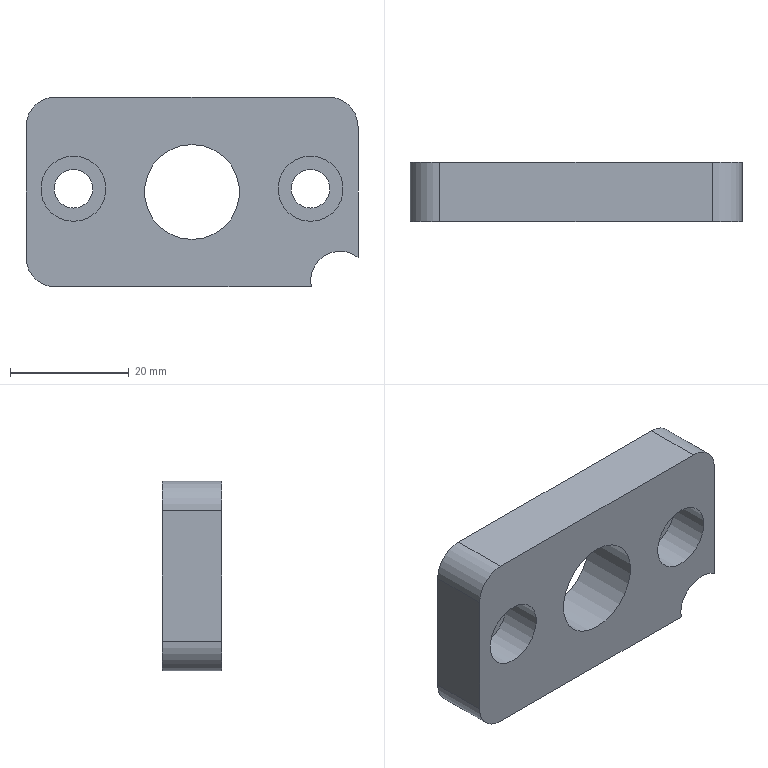Part | STEP file | B-PLATE-INSERT_id90_x_t | 1 solid | 17 faces | box 56 x 10 x 32 mm | volume 13802 mm3 | cylinder 9 | plane 8 | commonest cylinder face diameters 10 x4 6.5 x2 11 x2 16 x1
STEP:
#1=CARTESIAN_POINT('',(135.,-113.5,-39.958));
#2=VERTEX_POINT('',#1);
#3=CARTESIAN_POINT('',(135.,-113.5,-34.458));
#4=DIRECTION('',(0.,-1.,0.));
#5=DIRECTION('',(0.,0.,-1.));
#6=AXIS2_PLACEMENT_3D('',#3,#4,#5);
#7=CIRCLE('',#6,5.5);
#8=EDGE_CURVE('',#2,#2,#7,.T.);
#9=ORIENTED_EDGE('',*,*,#8,.F.);
#10=EDGE_LOOP('',(#9));
#11=FACE_BOUND('',#10,.T.);
#12=CARTESIAN_POINT('',(135.,-120.5,-39.958));
#13=VERTEX_POINT('',#12);
#14=CARTESIAN_POINT('',(135.,-120.5,-34.458));
#15=DIRECTION('',(0.,1.,0.));
#16=DIRECTION('',(0.,0.,-1.));
#17=AXIS2_PLACEMENT_3D('',#14,#15,#16);
#18=CIRCLE('',#17,5.5);
#19=EDGE_CURVE('',#13,#13,#18,.T.);
#20=ORIENTED_EDGE('',*,*,#19,.F.);
#21=EDGE_LOOP('',(#20));
#22=FACE_BOUND('',#21,.T.);
#23=CARTESIAN_POINT('',(135.,-120.5,-34.458));
#24=DIRECTION('',(0.,-1.,0.));
#25=DIRECTION('',(0.,0.,-1.));
#26=AXIS2_PLACEMENT_3D('',#23,#24,#25);
#27=CYLINDRICAL_SURFACE('',#26,5.5);
#28=ADVANCED_FACE('',(#11,#22),#27,.F.);
#29=CARTESIAN_POINT('',(95.,-113.5,-39.958));
#30=VERTEX_POINT('',#29);
#31=CARTESIAN_POINT('',(95.,-113.5,-34.458));
#32=DIRECTION('',(0.,-1.,0.));
#33=DIRECTION('',(0.,0.,-1.));
#34=AXIS2_PLACEMENT_3D('',#31,#32,#33);
#35=CIRCLE('',#34,5.5);
#36=EDGE_CURVE('',#30,#30,#35,.T.);
#37=ORIENTED_EDGE('',*,*,#36,.F.);
#38=EDGE_LOOP('',(#37));
#39=FACE_BOUND('',#38,.T.);
#40=CARTESIAN_POINT('',(95.,-120.5,-39.958));
#41=VERTEX_POINT('',#40);
#42=CARTESIAN_POINT('',(95.,-120.5,-34.458));
#43=DIRECTION('',(0.,1.,0.));
#44=DIRECTION('',(0.,0.,-1.));
#45=AXIS2_PLACEMENT_3D('',#42,#43,#44);
#46=CIRCLE('',#45,5.5);
#47=EDGE_CURVE('',#41,#41,#46,.T.);
#48=ORIENTED_EDGE('',*,*,#47,.F.);
#49=EDGE_LOOP('',(#48));
#50=FACE_BOUND('',#49,.T.);
#51=CARTESIAN_POINT('',(95.,-120.5,-34.458));
#52=DIRECTION('',(0.,-1.,0.));
#53=DIRECTION('',(0.,0.,-1.));
#54=AXIS2_PLACEMENT_3D('',#51,#52,#53);
#55=CYLINDRICAL_SURFACE('',#54,5.5);
#56=ADVANCED_FACE('',(#39,#50),#55,.F.);
#57=CARTESIAN_POINT('',(115.,-120.5,-43.));
#58=VERTEX_POINT('',#57);
#59=CARTESIAN_POINT('',(115.,-120.5,-35.));
#60=DIRECTION('',(0.,-1.,0.));
#61=DIRECTION('',(0.,0.,-1.));
#62=AXIS2_PLACEMENT_3D('',#59,#60,#61);
#63=CIRCLE('',#62,8.);
#64=EDGE_CURVE('',#58,#58,#63,.T.);
#65=ORIENTED_EDGE('',*,*,#64,.F.);
#66=EDGE_LOOP('',(#65));
#67=FACE_BOUND('',#66,.T.);
#68=ORIENTED_EDGE('',*,*,#47,.T.);
#69=EDGE_LOOP('',(#68));
#70=FACE_BOUND('',#69,.T.);
#71=ORIENTED_EDGE('',*,*,#19,.T.);
#72=EDGE_LOOP('',(#71));
#73=FACE_BOUND('',#72,.T.);
#74=CARTESIAN_POINT('',(87.,-120.5,-46.));
#75=VERTEX_POINT('',#74);
#76=CARTESIAN_POINT('',(87.,-120.5,-24.));
#77=VERTEX_POINT('',#76);
#78=CARTESIAN_POINT('',(87.,-120.5,-24.));
#79=DIRECTION('',(0.,0.,1.));
#80=VECTOR('',#79,1.);
#81=LINE('',#78,#80);
#82=EDGE_CURVE('',#75,#77,#81,.T.);
#83=ORIENTED_EDGE('',*,*,#82,.F.);
#84=CARTESIAN_POINT('',(92.,-120.5,-51.));
#85=VERTEX_POINT('',#84);
#86=CARTESIAN_POINT('',(92.,-120.5,-46.));
#87=DIRECTION('',(0.,1.,0.));
#88=DIRECTION('',(0.,0.,-1.));
#89=AXIS2_PLACEMENT_3D('',#86,#87,#88);
#90=CIRCLE('',#89,5.);
#91=EDGE_CURVE('',#85,#75,#90,.T.);
#92=ORIENTED_EDGE('',*,*,#91,.F.);
#93=CARTESIAN_POINT('',(135.101,-120.5,-51.));
#94=VERTEX_POINT('',#93);
#95=CARTESIAN_POINT('',(92.,-120.5,-51.));
#96=DIRECTION('',(-1.,0.,0.));
#97=VECTOR('',#96,1.);
#98=LINE('',#95,#97);
#99=EDGE_CURVE('',#94,#85,#98,.T.);
#100=ORIENTED_EDGE('',*,*,#99,.F.);
#101=CARTESIAN_POINT('',(143.,-120.5,-46.));
#102=VERTEX_POINT('',#101);
#103=CARTESIAN_POINT('',(140.,-120.5,-50.));
#104=DIRECTION('',(0.,1.,0.));
#105=DIRECTION('',(0.,0.,-1.));
#106=AXIS2_PLACEMENT_3D('',#103,#104,#105);
#107=CIRCLE('',#106,5.);
#108=EDGE_CURVE('',#94,#102,#107,.T.);
#109=ORIENTED_EDGE('',*,*,#108,.T.);
#110=CARTESIAN_POINT('',(143.,-120.5,-24.));
#111=VERTEX_POINT('',#110);
#112=CARTESIAN_POINT('',(143.,-120.5,-46.));
#113=DIRECTION('',(0.,0.,-1.));
#114=VECTOR('',#113,1.);
#115=LINE('',#112,#114);
#116=EDGE_CURVE('',#111,#102,#115,.T.);
#117=ORIENTED_EDGE('',*,*,#116,.F.);
#118=CARTESIAN_POINT('',(138.,-120.5,-19.));
#119=VERTEX_POINT('',#118);
#120=CARTESIAN_POINT('',(138.,-120.5,-24.));
#121=DIRECTION('',(0.,1.,0.));
#122=DIRECTION('',(0.,0.,-1.));
#123=AXIS2_PLACEMENT_3D('',#120,#121,#122);
#124=CIRCLE('',#123,5.);
#125=EDGE_CURVE('',#119,#111,#124,.T.);
#126=ORIENTED_EDGE('',*,*,#125,.F.);
#127=CARTESIAN_POINT('',(92.,-120.5,-19.));
#128=VERTEX_POINT('',#127);
#129=CARTESIAN_POINT('',(138.,-120.5,-19.));
#130=DIRECTION('',(1.,0.,0.));
#131=VECTOR('',#130,1.);
#132=LINE('',#129,#131);
#133=EDGE_CURVE('',#128,#119,#132,.T.);
#134=ORIENTED_EDGE('',*,*,#133,.F.);
#135=CARTESIAN_POINT('',(92.,-120.5,-24.));
#136=DIRECTION('',(0.,1.,0.));
#137=DIRECTION('',(0.,0.,-1.));
#138=AXIS2_PLACEMENT_3D('',#135,#136,#137);
#139=CIRCLE('',#138,5.);
#140=EDGE_CURVE('',#77,#128,#139,.T.);
#141=ORIENTED_EDGE('',*,*,#140,.F.);
#142=EDGE_LOOP('',(#83,#92,#100,#109,#117,#126,#134,#141));
#143=FACE_BOUND('',#142,.T.);
#144=CARTESIAN_POINT('',(-80.,-120.5,-43.));
#145=DIRECTION('',(0.,-1.,0.));
#146=DIRECTION('',(0.,0.,-1.));
#147=AXIS2_PLACEMENT_3D('',#144,#145,#146);
#148=PLANE('',#147);
#149=ADVANCED_FACE('',(#67,#70,#73,#143),#148,.T.);
#150=CARTESIAN_POINT('',(135.,-113.5,-37.708));
#151=VERTEX_POINT('',#150);
#152=CARTESIAN_POINT('',(135.,-113.5,-34.458));
#153=DIRECTION('',(0.,1.,0.));
#154=DIRECTION('',(0.,0.,-1.));
#155=AXIS2_PLACEMENT_3D('',#152,#153,#154);
#156=CIRCLE('',#155,3.25);
#157=EDGE_CURVE('',#151,#151,#156,.T.);
#158=ORIENTED_EDGE('',*,*,#157,.T.);
#159=EDGE_LOOP('',(#158));
#160=FACE_BOUND('',#159,.T.);
#161=ORIENTED_EDGE('',*,*,#8,.T.);
#162=EDGE_LOOP('',(#161));
#163=FACE_BOUND('',#162,.T.);
#164=CARTESIAN_POINT('',(-200.,-113.5,-275.));
#165=DIRECTION('',(0.,-1.,0.));
#166=DIRECTION('',(0.,0.,-1.));
#167=AXIS2_PLACEMENT_3D('',#164,#165,#166);
#168=PLANE('',#167);
#169=ADVANCED_FACE('',(#160,#163),#168,.T.);
#170=CARTESIAN_POINT('',(95.,-113.5,-37.708));
#171=VERTEX_POINT('',#170);
#172=CARTESIAN_POINT('',(95.,-113.5,-34.458));
#173=DIRECTION('',(0.,1.,0.));
#174=DIRECTION('',(0.,0.,-1.));
#175=AXIS2_PLACEMENT_3D('',#172,#173,#174);
#176=CIRCLE('',#175,3.25);
#177=EDGE_CURVE('',#171,#171,#176,.T.);
#178=ORIENTED_EDGE('',*,*,#177,.T.);
#179=EDGE_LOOP('',(#178));
#180=FACE_BOUND('',#179,.T.);
#181=ORIENTED_EDGE('',*,*,#36,.T.);
#182=EDGE_LOOP('',(#181));
#183=FACE_BOUND('',#182,.T.);
#184=CARTESIAN_POINT('',(-200.,-113.5,-275.));
#185=DIRECTION('',(0.,-1.,0.));
#186=DIRECTION('',(0.,0.,-1.));
#187=AXIS2_PLACEMENT_3D('',#184,#185,#186);
#188=PLANE('',#187);
#189=ADVANCED_FACE('',(#180,#183),#188,.T.);
#190=CARTESIAN_POINT('',(87.,-110.5,-46.));
#191=VERTEX_POINT('',#190);
#192=CARTESIAN_POINT('',(87.,-110.5,-46.));
#193=DIRECTION('',(0.,-1.,0.));
#194=VECTOR('',#193,1.);
#195=LINE('',#192,#194);
#196=EDGE_CURVE('',#191,#75,#195,.T.);
#197=ORIENTED_EDGE('',*,*,#196,.F.);
#198=CARTESIAN_POINT('',(92.,-110.5,-51.));
#199=VERTEX_POINT('',#198);
#200=CARTESIAN_POINT('',(92.,-110.5,-46.));
#201=DIRECTION('',(0.,-1.,0.));
#202=DIRECTION('',(0.,0.,-1.));
#203=AXIS2_PLACEMENT_3D('',#200,#201,#202);
#204=CIRCLE('',#203,5.);
#205=EDGE_CURVE('',#191,#199,#204,.T.);
#206=ORIENTED_EDGE('',*,*,#205,.T.);
#207=CARTESIAN_POINT('',(92.,-110.5,-51.));
#208=DIRECTION('',(0.,1.,0.));
#209=VECTOR('',#208,1.);
#210=LINE('',#207,#209);
#211=EDGE_CURVE('',#85,#199,#210,.T.);
#212=ORIENTED_EDGE('',*,*,#211,.F.);
#213=ORIENTED_EDGE('',*,*,#91,.T.);
#214=EDGE_LOOP('',(#197,#206,#212,#213));
#215=FACE_OUTER_BOUND('',#214,.T.);
#216=CARTESIAN_POINT('',(92.,-110.5,-46.));
#217=DIRECTION('',(0.,-1.,0.));
#218=DIRECTION('',(0.,0.,-1.));
#219=AXIS2_PLACEMENT_3D('',#216,#217,#218);
#220=CYLINDRICAL_SURFACE('',#219,5.);
#221=ADVANCED_FACE('',(#215),#220,.T.);
#222=ORIENTED_EDGE('',*,*,#211,.T.);
#223=CARTESIAN_POINT('',(135.101,-110.5,-51.));
#224=VERTEX_POINT('',#223);
#225=CARTESIAN_POINT('',(-200.,-110.5,-51.));
#226=DIRECTION('',(1.,0.,0.));
#227=VECTOR('',#226,1.);
#228=LINE('',#225,#227);
#229=EDGE_CURVE('',#199,#224,#228,.T.);
#230=ORIENTED_EDGE('',*,*,#229,.T.);
#231=CARTESIAN_POINT('',(135.101,-110.5,-51.));
#232=DIRECTION('',(0.,-1.,0.));
#233=VECTOR('',#232,1.);
#234=LINE('',#231,#233);
#235=EDGE_CURVE('',#224,#94,#234,.T.);
#236=ORIENTED_EDGE('',*,*,#235,.T.);
#237=ORIENTED_EDGE('',*,*,#99,.T.);
#238=EDGE_LOOP('',(#222,#230,#236,#237));
#239=FACE_OUTER_BOUND('',#238,.T.);
#240=CARTESIAN_POINT('',(92.,-110.5,-51.));
#241=DIRECTION('',(0.,0.,-1.));
#242=DIRECTION('',(-1.,0.,0.));
#243=AXIS2_PLACEMENT_3D('',#240,#241,#242);
#244=PLANE('',#243);
#245=ADVANCED_FACE('',(#239),#244,.T.);
#246=ORIENTED_EDGE('',*,*,#108,.F.);
#247=ORIENTED_EDGE('',*,*,#235,.F.);
#248=CARTESIAN_POINT('',(143.,-110.5,-46.));
#249=VERTEX_POINT('',#248);
#250=CARTESIAN_POINT('',(140.,-110.5,-50.));
#251=DIRECTION('',(0.,1.,0.));
#252=DIRECTION('',(0.,0.,-1.));
#253=AXIS2_PLACEMENT_3D('',#250,#251,#252);
#254=CIRCLE('',#253,5.);
#255=EDGE_CURVE('',#224,#249,#254,.T.);
#256=ORIENTED_EDGE('',*,*,#255,.T.);
#257=CARTESIAN_POINT('',(143.,-110.5,-46.));
#258=DIRECTION('',(0.,1.,0.));
#259=VECTOR('',#258,1.);
#260=LINE('',#257,#259);
#261=EDGE_CURVE('',#102,#249,#260,.T.);
#262=ORIENTED_EDGE('',*,*,#261,.F.);
#263=EDGE_LOOP('',(#246,#247,#256,#262));
#264=FACE_OUTER_BOUND('',#263,.T.);
#265=CARTESIAN_POINT('',(140.,-110.5,-50.));
#266=DIRECTION('',(0.,-1.,0.));
#267=DIRECTION('',(0.,0.,-1.));
#268=AXIS2_PLACEMENT_3D('',#265,#266,#267);
#269=CYLINDRICAL_SURFACE('',#268,5.);
#270=ADVANCED_FACE('',(#264),#269,.F.);
#271=ORIENTED_EDGE('',*,*,#261,.T.);
#272=CARTESIAN_POINT('',(143.,-110.5,-24.));
#273=VERTEX_POINT('',#272);
#274=CARTESIAN_POINT('',(143.,-110.5,-275.));
#275=DIRECTION('',(0.,0.,1.));
#276=VECTOR('',#275,1.);
#277=LINE('',#274,#276);
#278=EDGE_CURVE('',#249,#273,#277,.T.);
#279=ORIENTED_EDGE('',*,*,#278,.T.);
#280=CARTESIAN_POINT('',(143.,-110.5,-24.));
#281=DIRECTION('',(0.,1.,0.));
#282=VECTOR('',#281,1.);
#283=LINE('',#280,#282);
#284=EDGE_CURVE('',#111,#273,#283,.T.);
#285=ORIENTED_EDGE('',*,*,#284,.F.);
#286=ORIENTED_EDGE('',*,*,#116,.T.);
#287=EDGE_LOOP('',(#271,#279,#285,#286));
#288=FACE_OUTER_BOUND('',#287,.T.);
#289=CARTESIAN_POINT('',(143.,-110.5,-46.));
#290=DIRECTION('',(1.,0.,0.));
#291=DIRECTION('',(0.,0.,-1.));
#292=AXIS2_PLACEMENT_3D('',#289,#290,#291);
#293=PLANE('',#292);
#294=ADVANCED_FACE('',(#288),#293,.T.);
#295=ORIENTED_EDGE('',*,*,#284,.T.);
#296=CARTESIAN_POINT('',(138.,-110.5,-19.));
#297=VERTEX_POINT('',#296);
#298=CARTESIAN_POINT('',(138.,-110.5,-24.));
#299=DIRECTION('',(0.,-1.,0.));
#300=DIRECTION('',(0.,0.,-1.));
#301=AXIS2_PLACEMENT_3D('',#298,#299,#300);
#302=CIRCLE('',#301,5.);
#303=EDGE_CURVE('',#273,#297,#302,.T.);
#304=ORIENTED_EDGE('',*,*,#303,.T.);
#305=CARTESIAN_POINT('',(138.,-110.5,-19.));
#306=DIRECTION('',(0.,1.,0.));
#307=VECTOR('',#306,1.);
#308=LINE('',#305,#307);
#309=EDGE_CURVE('',#119,#297,#308,.T.);
#310=ORIENTED_EDGE('',*,*,#309,.F.);
#311=ORIENTED_EDGE('',*,*,#125,.T.);
#312=EDGE_LOOP('',(#295,#304,#310,#311));
#313=FACE_OUTER_BOUND('',#312,.T.);
#314=CARTESIAN_POINT('',(138.,-110.5,-24.));
#315=DIRECTION('',(0.,-1.,0.));
#316=DIRECTION('',(0.,0.,-1.));
#317=AXIS2_PLACEMENT_3D('',#314,#315,#316);
#318=CYLINDRICAL_SURFACE('',#317,5.);
#319=ADVANCED_FACE('',(#313),#318,.T.);
#320=ORIENTED_EDGE('',*,*,#309,.T.);
#321=CARTESIAN_POINT('',(92.,-110.5,-19.));
#322=VERTEX_POINT('',#321);
#323=CARTESIAN_POINT('',(-200.,-110.5,-19.));
#324=DIRECTION('',(-1.,0.,0.));
#325=VECTOR('',#324,1.);
#326=LINE('',#323,#325);
#327=EDGE_CURVE('',#297,#322,#326,.T.);
#328=ORIENTED_EDGE('',*,*,#327,.T.);
#329=CARTESIAN_POINT('',(92.,-110.5,-19.));
#330=DIRECTION('',(0.,1.,0.));
#331=VECTOR('',#330,1.);
#332=LINE('',#329,#331);
#333=EDGE_CURVE('',#128,#322,#332,.T.);
#334=ORIENTED_EDGE('',*,*,#333,.F.);
#335=ORIENTED_EDGE('',*,*,#133,.T.);
#336=EDGE_LOOP('',(#320,#328,#334,#335));
#337=FACE_OUTER_BOUND('',#336,.T.);
#338=CARTESIAN_POINT('',(138.,-110.5,-19.));
#339=DIRECTION('',(0.,0.,1.));
#340=DIRECTION('',(1.,0.,0.));
#341=AXIS2_PLACEMENT_3D('',#338,#339,#340);
#342=PLANE('',#341);
#343=ADVANCED_FACE('',(#337),#342,.T.);
#344=ORIENTED_EDGE('',*,*,#333,.T.);
#345=CARTESIAN_POINT('',(87.,-110.5,-24.));
#346=VERTEX_POINT('',#345);
#347=CARTESIAN_POINT('',(92.,-110.5,-24.));
#348=DIRECTION('',(0.,-1.,0.));
#349=DIRECTION('',(0.,0.,-1.));
#350=AXIS2_PLACEMENT_3D('',#347,#348,#349);
#351=CIRCLE('',#350,5.);
#352=EDGE_CURVE('',#322,#346,#351,.T.);
#353=ORIENTED_EDGE('',*,*,#352,.T.);
#354=CARTESIAN_POINT('',(87.,-110.5,-24.));
#355=DIRECTION('',(0.,1.,0.));
#356=VECTOR('',#355,1.);
#357=LINE('',#354,#356);
#358=EDGE_CURVE('',#77,#346,#357,.T.);
#359=ORIENTED_EDGE('',*,*,#358,.F.);
#360=ORIENTED_EDGE('',*,*,#140,.T.);
#361=EDGE_LOOP('',(#344,#353,#359,#360));
#362=FACE_OUTER_BOUND('',#361,.T.);
#363=CARTESIAN_POINT('',(92.,-110.5,-24.));
#364=DIRECTION('',(0.,-1.,0.));
#365=DIRECTION('',(0.,0.,-1.));
#366=AXIS2_PLACEMENT_3D('',#363,#364,#365);
#367=CYLINDRICAL_SURFACE('',#366,5.);
#368=ADVANCED_FACE('',(#362),#367,.T.);
#369=ORIENTED_EDGE('',*,*,#358,.T.);
#370=CARTESIAN_POINT('',(87.,-110.5,-275.));
#371=DIRECTION('',(0.,0.,-1.));
#372=VECTOR('',#371,1.);
#373=LINE('',#370,#372);
#374=EDGE_CURVE('',#346,#191,#373,.T.);
#375=ORIENTED_EDGE('',*,*,#374,.T.);
#376=ORIENTED_EDGE('',*,*,#196,.T.);
#377=ORIENTED_EDGE('',*,*,#82,.T.);
#378=EDGE_LOOP('',(#369,#375,#376,#377));
#379=FACE_OUTER_BOUND('',#378,.T.);
#380=CARTESIAN_POINT('',(87.,-110.5,-24.));
#381=DIRECTION('',(-1.,0.,0.));
#382=DIRECTION('',(0.,0.,1.));
#383=AXIS2_PLACEMENT_3D('',#380,#381,#382);
#384=PLANE('',#383);
#385=ADVANCED_FACE('',(#379),#384,.T.);
#386=CARTESIAN_POINT('',(135.,-110.5,-37.708));
#387=VERTEX_POINT('',#386);
#388=CARTESIAN_POINT('',(135.,-110.5,-34.458));
#389=DIRECTION('',(0.,1.,0.));
#390=DIRECTION('',(0.,0.,-1.));
#391=AXIS2_PLACEMENT_3D('',#388,#389,#390);
#392=CIRCLE('',#391,3.25);
#393=EDGE_CURVE('',#387,#387,#392,.T.);
#394=ORIENTED_EDGE('',*,*,#393,.T.);
#395=EDGE_LOOP('',(#394));
#396=FACE_BOUND('',#395,.T.);
#397=ORIENTED_EDGE('',*,*,#157,.F.);
#398=EDGE_LOOP('',(#397));
#399=FACE_BOUND('',#398,.T.);
#400=CARTESIAN_POINT('',(135.,-120.5,-34.458));
#401=DIRECTION('',(0.,-1.,0.));
#402=DIRECTION('',(0.,0.,-1.));
#403=AXIS2_PLACEMENT_3D('',#400,#401,#402);
#404=CYLINDRICAL_SURFACE('',#403,3.25);
#405=ADVANCED_FACE('',(#396,#399),#404,.F.);
#406=CARTESIAN_POINT('',(95.,-110.5,-37.708));
#407=VERTEX_POINT('',#406);
#408=CARTESIAN_POINT('',(95.,-110.5,-34.458));
#409=DIRECTION('',(0.,1.,0.));
#410=DIRECTION('',(0.,0.,-1.));
#411=AXIS2_PLACEMENT_3D('',#408,#409,#410);
#412=CIRCLE('',#411,3.25);
#413=EDGE_CURVE('',#407,#407,#412,.T.);
#414=ORIENTED_EDGE('',*,*,#413,.T.);
#415=EDGE_LOOP('',(#414));
#416=FACE_BOUND('',#415,.T.);
#417=ORIENTED_EDGE('',*,*,#177,.F.);
#418=EDGE_LOOP('',(#417));
#419=FACE_BOUND('',#418,.T.);
#420=CARTESIAN_POINT('',(95.,-120.5,-34.458));
#421=DIRECTION('',(0.,-1.,0.));
#422=DIRECTION('',(0.,0.,-1.));
#423=AXIS2_PLACEMENT_3D('',#420,#421,#422);
#424=CYLINDRICAL_SURFACE('',#423,3.25);
#425=ADVANCED_FACE('',(#416,#419),#424,.F.);
#426=CARTESIAN_POINT('',(115.,-110.5,-43.));
#427=VERTEX_POINT('',#426);
#428=CARTESIAN_POINT('',(115.,-110.5,-35.));
#429=DIRECTION('',(0.,-1.,0.));
#430=DIRECTION('',(0.,0.,-1.));
#431=AXIS2_PLACEMENT_3D('',#428,#429,#430);
#432=CIRCLE('',#431,8.);
#433=EDGE_CURVE('',#427,#427,#432,.T.);
#434=ORIENTED_EDGE('',*,*,#433,.T.);
#435=EDGE_LOOP('',(#434));
#436=FACE_BOUND('',#435,.T.);
#437=ORIENTED_EDGE('',*,*,#413,.F.);
#438=EDGE_LOOP('',(#437));
#439=FACE_BOUND('',#438,.T.);
#440=ORIENTED_EDGE('',*,*,#393,.F.);
#441=EDGE_LOOP('',(#440));
#442=FACE_BOUND('',#441,.T.);
#443=ORIENTED_EDGE('',*,*,#352,.F.);
#444=ORIENTED_EDGE('',*,*,#327,.F.);
#445=ORIENTED_EDGE('',*,*,#303,.F.);
#446=ORIENTED_EDGE('',*,*,#278,.F.);
#447=ORIENTED_EDGE('',*,*,#255,.F.);
#448=ORIENTED_EDGE('',*,*,#229,.F.);
#449=ORIENTED_EDGE('',*,*,#205,.F.);
#450=ORIENTED_EDGE('',*,*,#374,.F.);
#451=EDGE_LOOP('',(#443,#444,#445,#446,#447,#448,#449,#450));
#452=FACE_BOUND('',#451,.T.);
#453=CARTESIAN_POINT('',(-200.,-110.5,-275.));
#454=DIRECTION('',(0.,-1.,0.));
#455=DIRECTION('',(0.,0.,-1.));
#456=AXIS2_PLACEMENT_3D('',#453,#454,#455);
#457=PLANE('',#456);
#458=ADVANCED_FACE('',(#436,#439,#442,#452),#457,.F.);
#459=ORIENTED_EDGE('',*,*,#64,.T.);
#460=EDGE_LOOP('',(#459));
#461=FACE_BOUND('',#460,.T.);
#462=ORIENTED_EDGE('',*,*,#433,.F.);
#463=EDGE_LOOP('',(#462));
#464=FACE_BOUND('',#463,.T.);
#465=CARTESIAN_POINT('',(115.,-231.55,-35.));
#466=DIRECTION('',(0.,-1.,0.));
#467=DIRECTION('',(0.,0.,-1.));
#468=AXIS2_PLACEMENT_3D('',#465,#466,#467);
#469=CYLINDRICAL_SURFACE('',#468,8.);
#470=ADVANCED_FACE('',(#461,#464),#469,.F.);
#471=CLOSED_SHELL('',(#28,#56,#149,#169,#189,#221,#245,#270,#294,#319,#343,#368,#385,#405,#425,#458,#470));
#472=MANIFOLD_SOLID_BREP('',#471);
#473=(LENGTH_UNIT()NAMED_UNIT(*)SI_UNIT(.MILLI.,.METRE.));
#474=UNCERTAINTY_MEASURE_WITH_UNIT(LENGTH_MEASURE(0.00002),#473,'','');
#475=(NAMED_UNIT(*)PLANE_ANGLE_UNIT()SI_UNIT($,.RADIAN.));
#476=PLANE_ANGLE_MEASURE_WITH_UNIT(PLANE_ANGLE_MEASURE(0.01745),#475);
#477=DIMENSIONAL_EXPONENTS(0.,0.,0.,0.,0.,0.,0.);
#478=(CONVERSION_BASED_UNIT('DEGREE',#476)NAMED_UNIT(#477)PLANE_ANGLE_UNIT());
#479=(NAMED_UNIT(*)SI_UNIT($,.STERADIAN.)SOLID_ANGLE_UNIT());
#480=(GEOMETRIC_REPRESENTATION_CONTEXT(3)GLOBAL_UNCERTAINTY_ASSIGNED_CONTEXT((#474))GLOBAL_UNIT_ASSIGNED_CONTEXT((#473,#478,#479))REPRESENTATION_CONTEXT('',''));
#481=ADVANCED_BREP_SHAPE_REPRESENTATION('',(#472),#480);